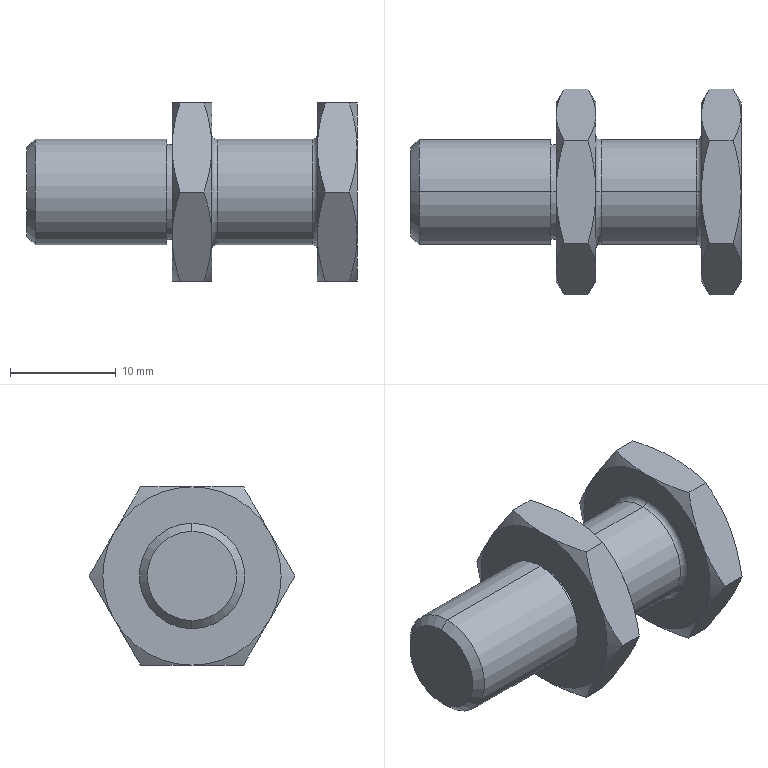Part | STEP file | Part 66 | 1 solid | 54 faces | box 31.25 x 19.486 x 16.875 mm | volume 3681 mm3 | cone 26 | plane 18 | cylinder 6 | torus 4 | commonest cylinder face diameters 10 x4 9 x2